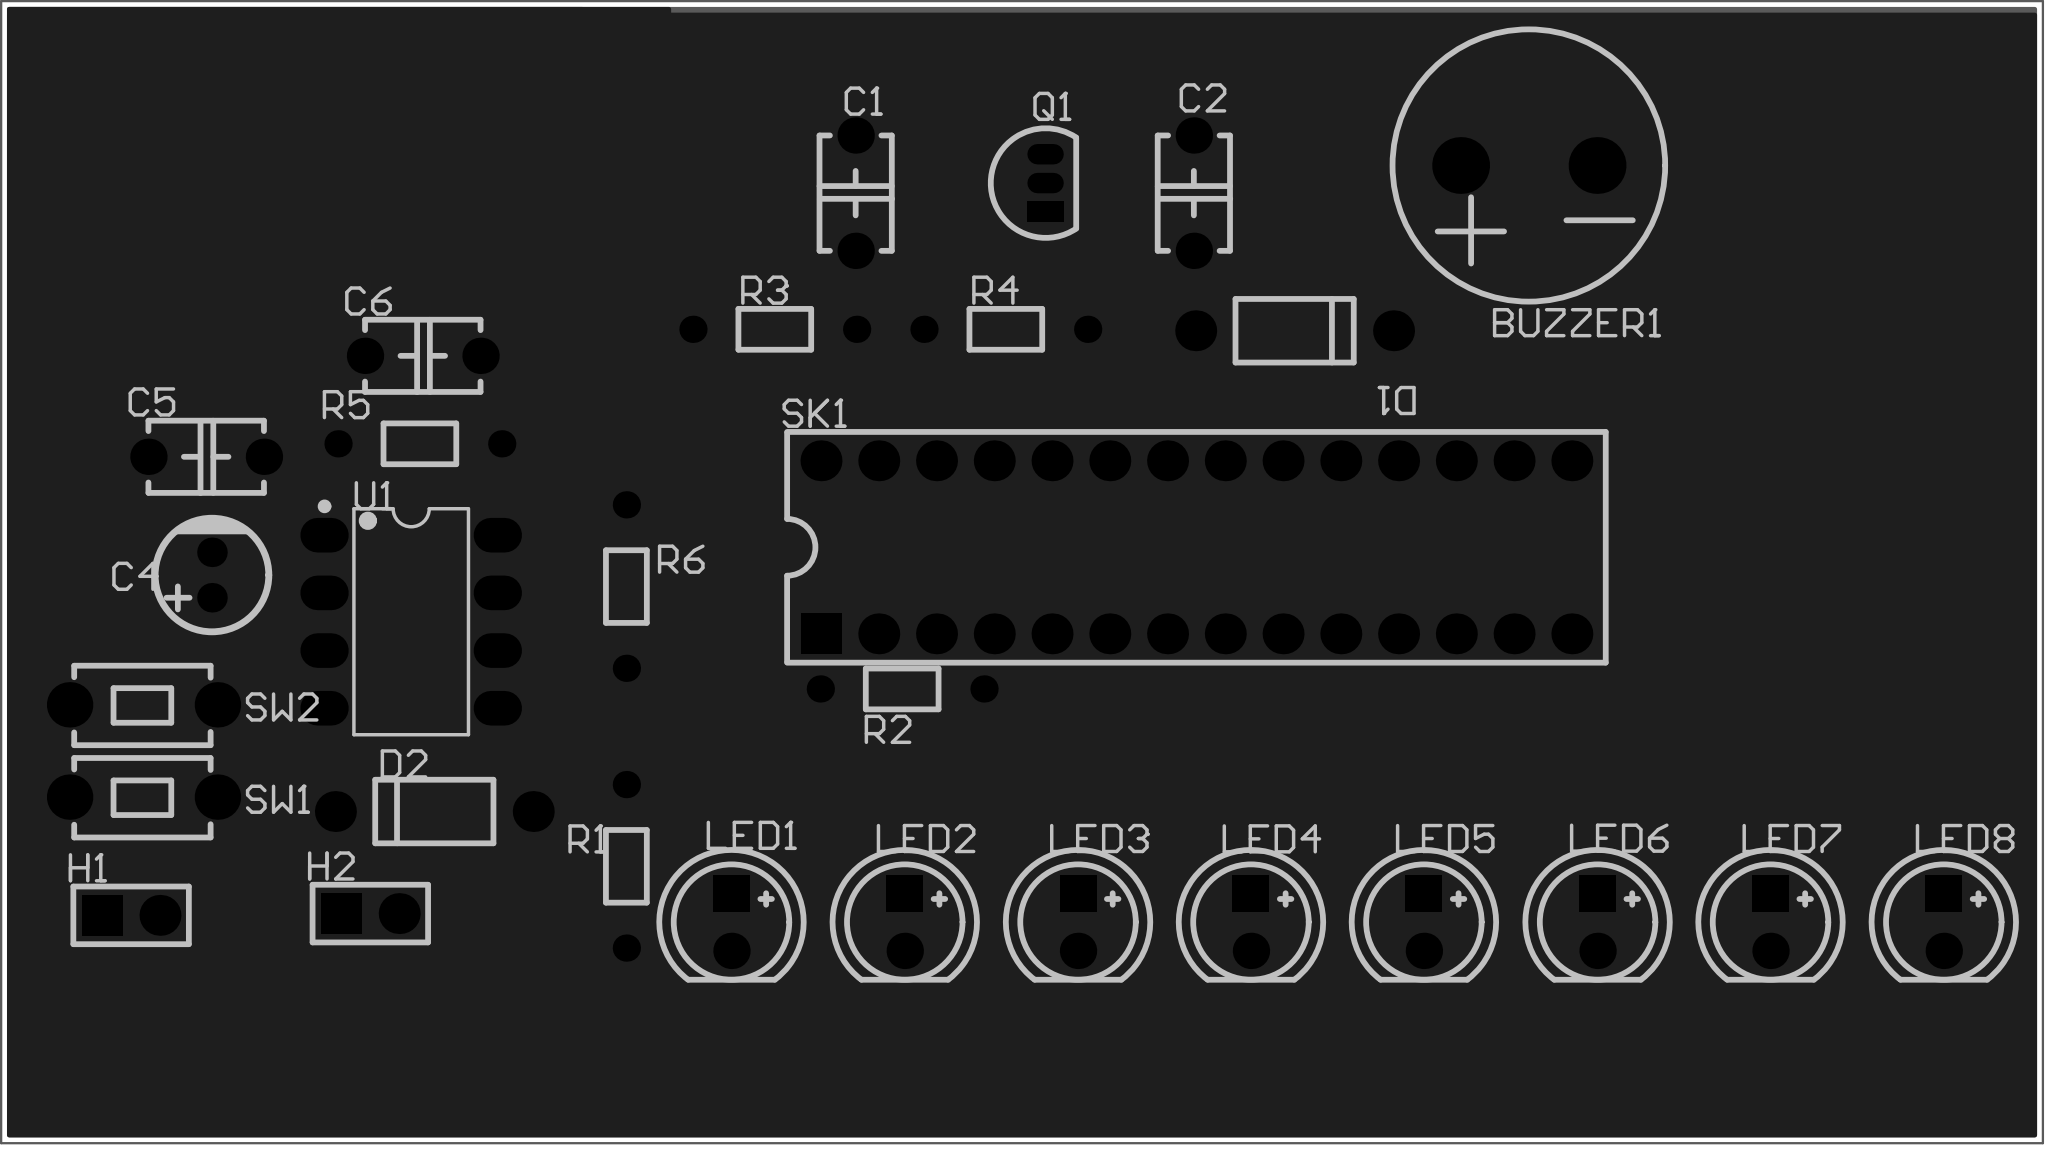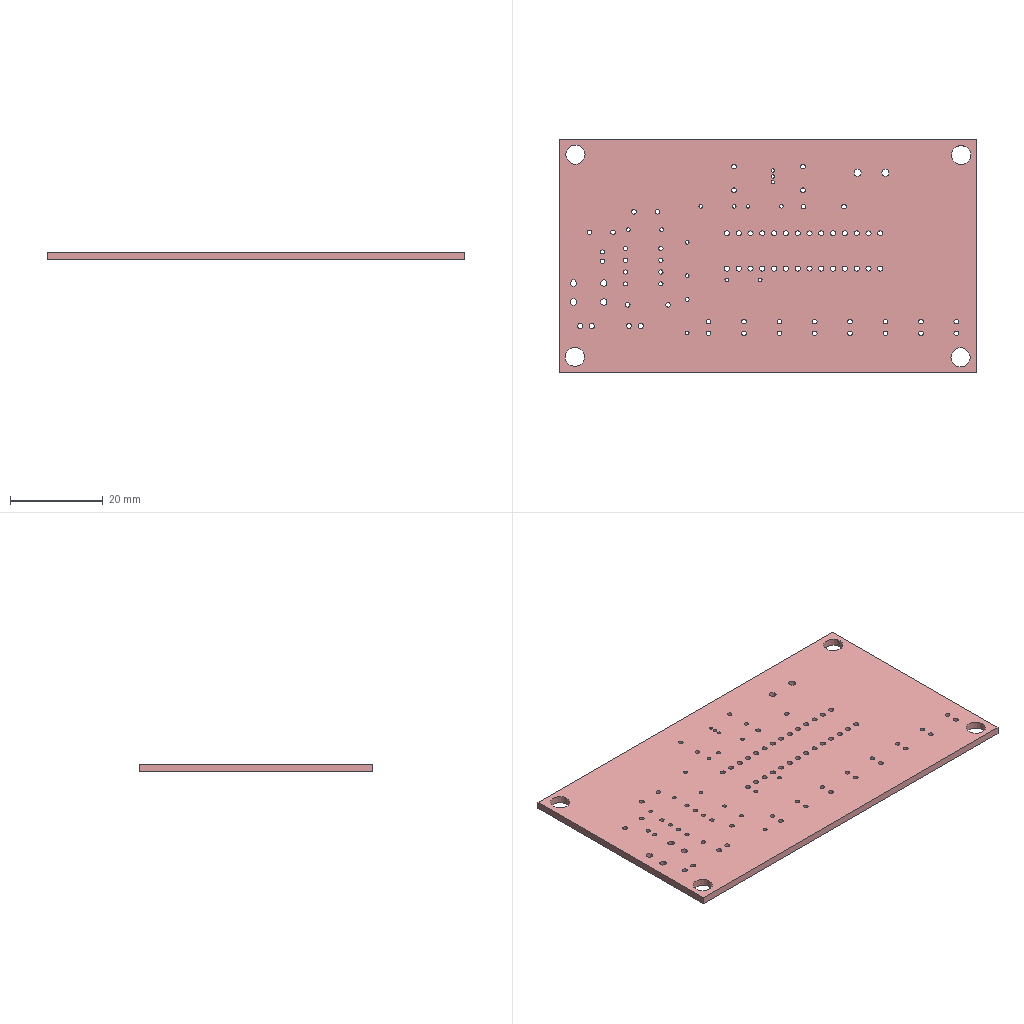Circuit board layout | Altium Designer | box 89.8 x 50.3 x 1.6 mm
Layer stack:
# Altium Designer layer stack of  (unit mm; dielectric type: 0 none, 1 core, 2 prepreg, 3 surface material)
index,name,kind,layer,copper_thickness_mm,dielectric_type,dielectric_thickness_mm,dielectric_material,dielectric_constant
0,Top Paste Mask Layer,other,,,,,,
1,Top Silkscreen Layer,other,,,,,,
2,Top Solder Mask Layer,dielectric,,,3,0.01,,3.3
3,Top Layer,copper,Top Layer,0.035,,,,
4,Dielectric1,dielectric,,,3,1.51,FR4,4.5
5,Bottom Layer,copper,Bottom Layer,0.035,,,,
6,Bottom Solder Mask Layer,dielectric,,,3,0.01,,3.3
7,Bottom Silkscreen Layer,other,,,,,,
8,Bottom Paste Mask Layer,other,,,,,,
# drill layer pairs: low layer,high layer
drill_pair,Top Layer,Bottom Layer
Part placement:
Designator,Comment,Layer,Footprint,Center-X(mm),Center-Y(mm),Rotation
BUZZER1,buzzer,TopLayer,BUZ-TH_BD12.0-P6.00-D0.9-RD,192.024,134.493,180
C1,0.1uF,TopLayer,CAP-TH_L5.1-W3.2-P5.08-D0.50,162.419,133.275,90
C2,0.047uF,TopLayer,CAP-TH_L5.1-W3.2-P5.08-D0.50,177.292,133.275,90
C4,10uF,TopLayer,CAP-TH_BD5.0-P2.00-D0.8-FD-10UF50VC110GL,134.112,116.459,90
C5,10nF,TopLayer,CAP-TH_L5.1-W3.2-P5.08-D0.50,133.858,121.666,0
D1,,TopLayer,DO_1N4007,181.724,127.216,180
D2,,TopLayer,DO_1N4007,143.891,106.045,0
H1,,TopLayer,HDR-TH_2P-P2.54-V-M-1,130.556,101.473,0
H2,,TopLayer,HDR-TH_2P-P2.54-V-M-1,141.076,101.551,0
LED1,,TopLayer,LED-TH_5mm,156.958,101.178,270
LED2,,TopLayer,LED-TH_5mm,164.578,101.178,270
LED3,,TopLayer,LED-TH_5mm,172.198,101.178,270
LED4,,TopLayer,LED-TH_5mm,179.804,101.178,270
LED5,,TopLayer,LED-TH_5mm,187.409,101.178,270
LED6,,TopLayer,LED-TH_5mm,195.046,101.178,270
LED7,,TopLayer,LED-TH_5mm,202.651,101.178,270
LED8,,TopLayer,LED-TH_5mm,210.271,101.178,270
Q1,,TopLayer,S8050_TO_92,170.772,133.719,90
R1,1kΩ,TopLayer,Res_1/8W,152.336,103.632,270
R2,22kΩ,TopLayer,Res_1/8W,164.465,111.443,180
R3,100kΩ,TopLayer,Res_1/8W,158.863,127.279,0
R4,100kΩ,TopLayer,Res_1/8W,169.024,127.279,0
R5,10kΩ,TopLayer,Res_1/8W,143.256,122.237,0
R6,10kΩ,TopLayer,Res_1/8W,152.337,115.951,90
SK1,X5621WV-2x14-C762D1000-1000,TopLayer,DIP-28_L35.6-W10.2-P2.54-LS7.6-BL,177.405,117.68,0
SW1,,TopLayer,Key_TH_3.5x6x4.3,131.102,106.68,0
SW2,,TopLayer,Key_TH_3.5x6x4.3,131.102,110.744,0
U1,NE555,TopLayer,DIP-8_L9.8-W6.4-P2.54-LS7.6-BL,142.873,114.403,270
C6,10nF,TopLayer,CAP-TH_L5.1-W3.2-P5.08-D0.50,143.383,126.111,0
Pad and via stacks:
# Altium Designer via and pad stacks of  (unit mm). Each distinct definition once, with the count of objects using it.
# via: kind,start_layer,end_layer,hole_mm,diameter_mm,mode(0 simple;1 top-mid-bottom;2 full stack),diameter_per_layer,count,example_net
# pad: kind,layer,hole_mm,hole_type(0 round;1 square;2 slot),plating,top_size,top_shape(1 round;2 rect;3 octagon;9 rounded rect),mid_size,bottom_size,mode,footprint,size_per_layer,count,example
pad,Multi-Layer,1.5,0,plated,2.5x2.5,1,2.5x2.5,2.5x2.5,0,BUZ-TH_BD12.0-P6.00-D0.9-RD,,2,BUZZER1.1
pad,Multi-Layer,1,0,plated,1.6x1.6,1,1.6x1.6,1.6x1.6,0,CAP-TH_L5.1-W3.2-P5.08-D0.50,,8,C1.2
pad,Multi-Layer,0.9,0,plated,1.3x1.3,1,1.3x1.3,1.3x1.3,0,CAP-TH_BD5.0-P2.00-D0.8-FD-10UF50VC110GL,,2,C4.2
pad,Multi-Layer,1,0,plated,1.8x1.8,1,1.8x1.8,1.8x1.8,0,DO_1N4007,,4,D1.1
pad,Multi-Layer,1.1,0,plated,1.8x1.8,1,1.8x1.8,1.8x1.8,0,HDR-TH_2P-P2.54-V-M-1,,2,H1.2
pad,Multi-Layer,1.1,0,plated,1.8x1.8,2,1.8x1.8,1.8x1.8,0,HDR-TH_2P-P2.54-V-M-1,,2,H1.1
pad,Multi-Layer,1,0,plated,1.6x1.6,2,1.6x1.6,1.6x1.6,0,LED-TH_5mm,,8,LED1.1
pad,Multi-Layer,1,0,plated,1.6x1.6,1,1.6x1.6,1.6x1.6,0,LED-TH_5mm,,8,LED1.2
pad,Multi-Layer,0.701,0,plated,0.8992x1.6,2,0.8992x1.6,0.8992x1.6,0,S8050_TO_92,,1,Q1.1
pad,Multi-Layer,0.701,0,plated,0.8992x1.6,1,0.8992x1.6,0.8992x1.6,0,S8050_TO_92,,2,Q1.2
pad,Multi-Layer,0.8001,0,plated,1.199x1.199,1,1.199x1.199,1.199x1.199,0,Res_1/8W,,12,R1.1
pad,Multi-Layer,1.1,0,plated,1.8x1.8,2,1.8x1.8,1.8x1.8,0,DIP-28_L35.6-W10.2-P2.54-LS7.6-BL,,1,SK1.1
pad,Multi-Layer,1.1,0,plated,1.8x1.8,1,1.8x1.8,1.8x1.8,0,DIP-28_L35.6-W10.2-P2.54-LS7.6-BL,,27,SK1.2
pad,Multi-Layer,1.399,0,plated,1.999x1.999,1,1.999x1.999,1.999x1.999,0,Key_TH_3.5x6x4.3,,4,SW1.A
pad,Multi-Layer,0.9,0,plated,1.524x2.125,1,1.524x2.125,1.524x2.125,0,DIP-8_L9.8-W6.4-P2.54-LS7.6-BL,,8,U1.1
Copper pours:
name,layer,net,type(0 solid;1 hatched;2 none)
Top Layer-GND,Top Layer,GND,0
Top Layer-GND 1,Top Layer,GND,0
Bottom Layer-GND,Bottom Layer,GND,0
Bottom Layer-GND 1,Bottom Layer,GND,0
Design rules, without the lines most boards share:
# Altium Designer design rules of  (exported by Altium Designer, unit mm)
# columns: name | kind | enabled | priority | scope1 | scope2 | descriptor | typed fields (field=value)
creepage | 65 | enabled | 1 | All | All | Creepage Distance Constraint =(0mil) (All),(All) |